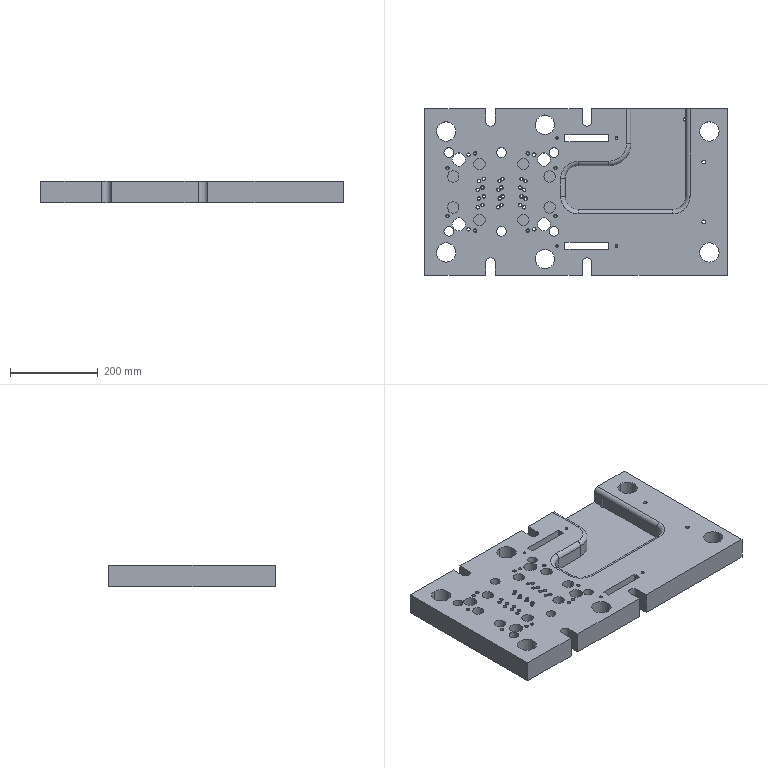Part | STEP file | 1 solid | 256 faces | box 690 x 380 x 50 mm | volume 10135272 mm3 | cylinder 119 | cone 91 | plane 42 | torus 4 | commonest cylinder face diameters 6.8 x32 1 x30 8.5 x10 22 x10 26 x8 44.01 x6